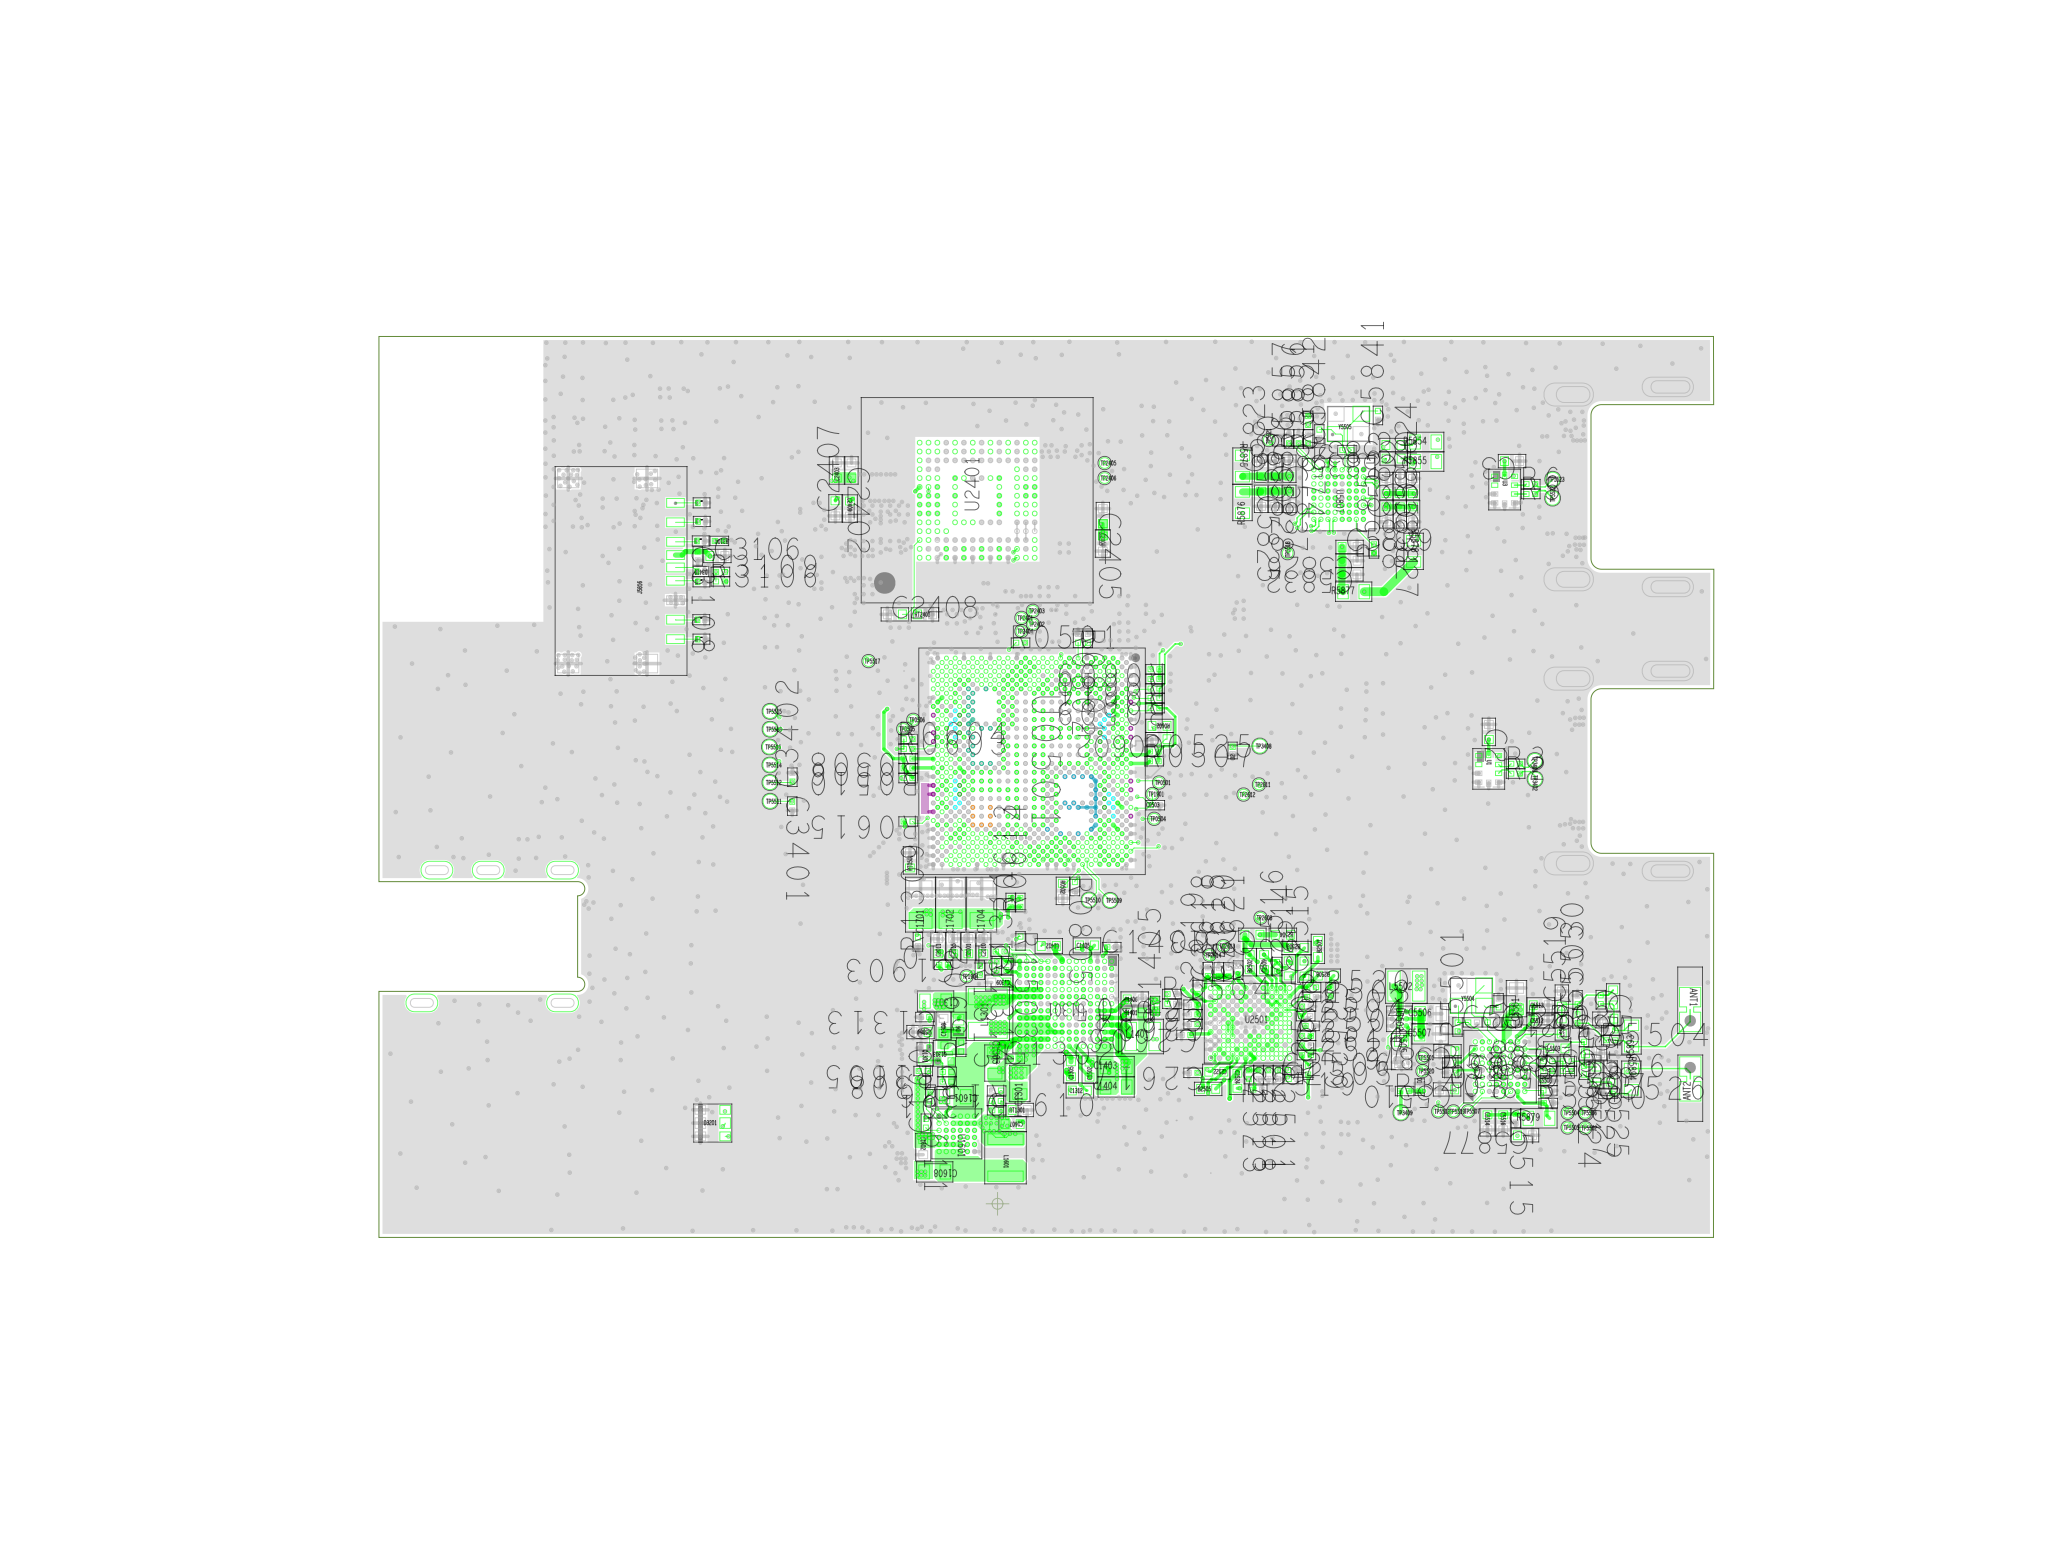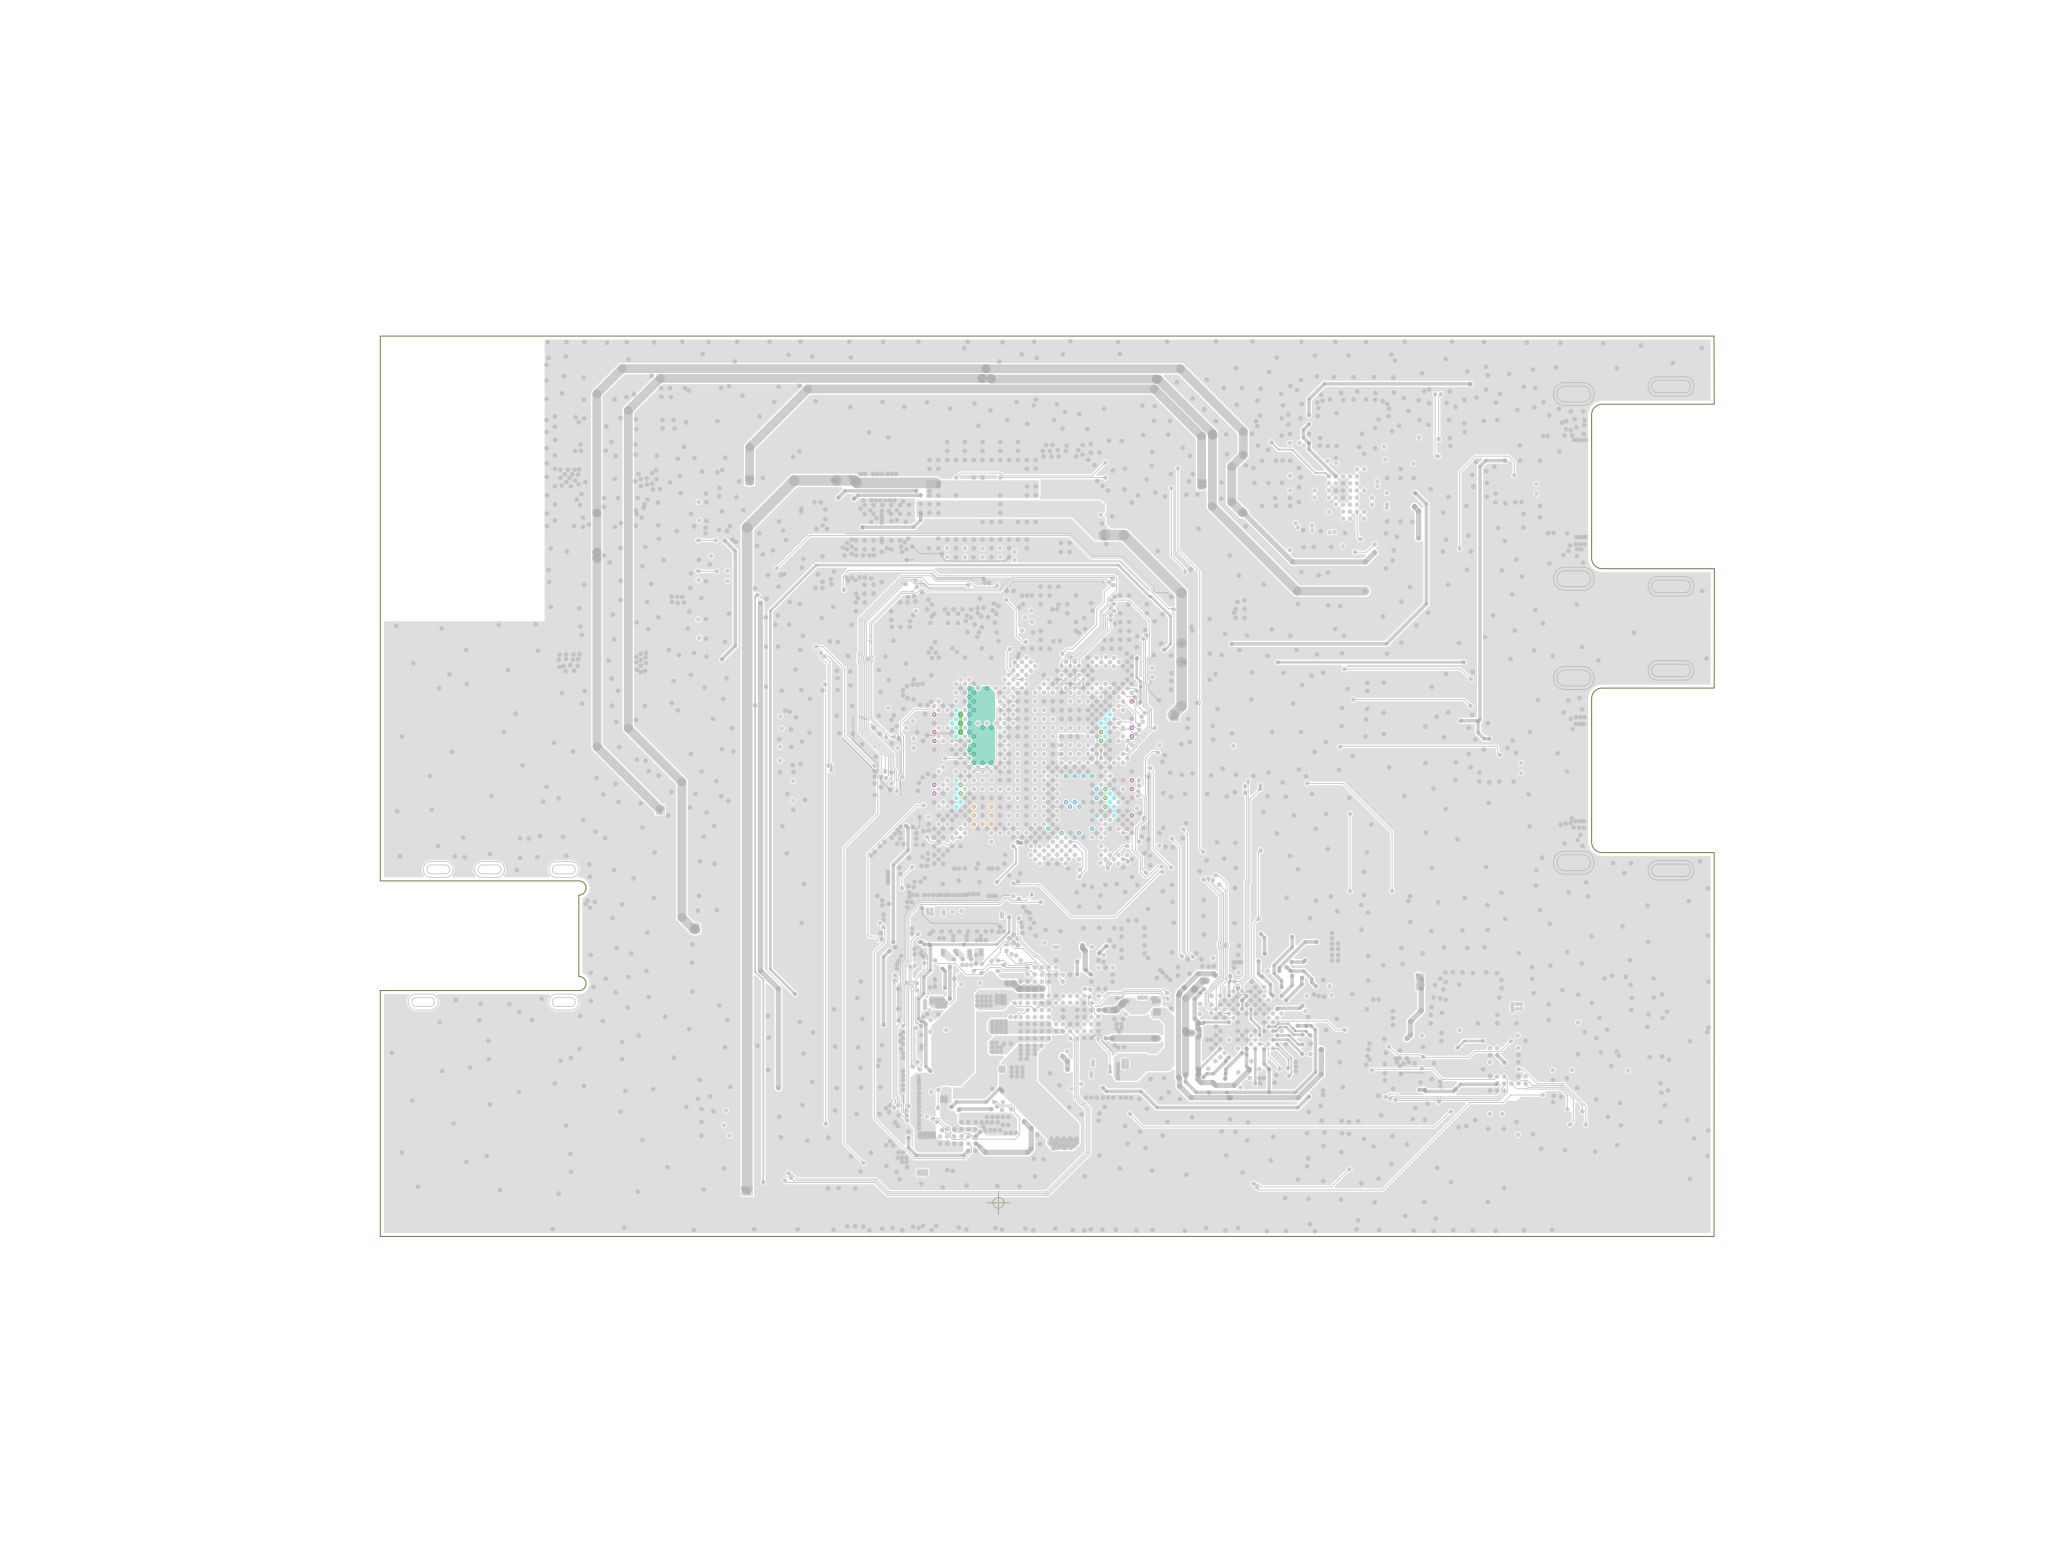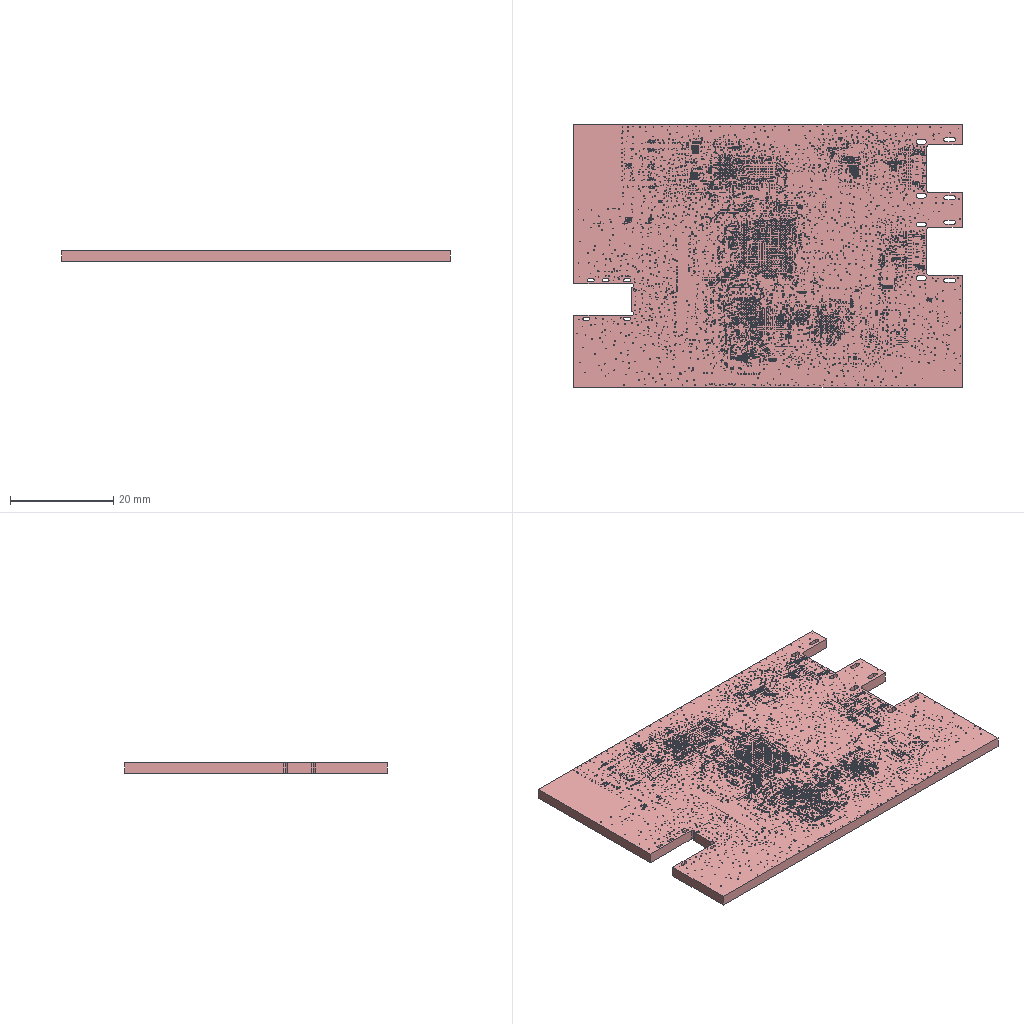Circuit board layout | Cadence Allegro | box 75.4 x 50.9 x 2.1 mm
Layer stack:
# Cadence Allegro layer stack of  (unit mm; from the constraint file cross-section; dielectric type: 0 not recorded (Allegro does not mark core vs prepreg), 3 surface material)
index,name,kind,layer,copper_thickness_mm,dielectric_type,dielectric_thickness_mm,dielectric_material,dielectric_constant
0,Top Surface,other,,,,,,
1,TOP,copper,TOP,0.0305,,,,
2,Dielectric1,dielectric,,,0,0.2032,FR-4,4.5
3,L2,copper,L2,0.0305,,,,
4,Dielectric2,dielectric,,,0,0.2032,FR-4,4.5
5,L3,copper,L3,0.0305,,,,
6,Dielectric3,dielectric,,,0,0.2032,FR-4,4.5
7,L4,copper,L4,0.0305,,,,
8,Dielectric4,dielectric,,,0,0.2032,FR-4,4.5
9,L5,copper,L5,0.0305,,,,
10,Dielectric5,dielectric,,,0,0.2032,FR-4,4.5
11,L6,copper,L6,0.0305,,,,
12,Dielectric6,dielectric,,,0,0.2032,FR-4,4.5
13,L7,copper,L7,0.0305,,,,
14,Dielectric7,dielectric,,,0,0.2032,FR-4,4.5
15,L8,copper,L8,0.0305,,,,
16,Dielectric8,dielectric,,,0,0.2032,FR-4,4.5
17,L9,copper,L9,0.0305,,,,
18,Dielectric9,dielectric,,,0,0.2032,FR-4,4.5
19,BOTTOM,copper,BOTTOM,0.0305,,,,
20,Bottom Surface,other,,,,,,
# drill layer pairs: low layer,high layer
drill_pair,TOP,BOTTOM
drill_pair,L5,BOTTOM
drill_pair,L9,BOTTOM
drill_pair,L2,BOTTOM
drill_pair,L3,BOTTOM
drill_pair,L4,BOTTOM
drill_pair,L6,BOTTOM
drill_pair,L8,BOTTOM
drill_pair,L7,BOTTOM
Part placement, first 475 of 804 lines:
REFDES,COMP_VALUE,SYM_NAME,SYM_X,SYM_Y,SYM_ROTATE,SYM_MIRROR
ANT1,818001475,PIN_ANT_818001475,39.13,11.5,270.000,NO
ANT2,818001475,PIN_ANT_818001475,39.14,6.53,90.000,NO
B301,HZ1005K102TF  1KOHM/100MHZ,FB0402,-23.65,9.9,180.000,YES
B302,HZ1005K102TF  1KOHM/100MHZ,FB0402,-29.6,20.55,270.000,YES
B303,MPZ1608S601AT  600OHM/100MHZ,FB0603_TDK,-24.55,20.25,180.000,YES
B304,HZ1005K102TF 1800ohm,FB0402,-19.1,16.93,180.000,YES
B306,HZ1005K102TF  1KOHM/100MHZ,FB0402,-19.56,15.72,270.000,YES
B2501,BLM15PD121SN1D 120OHM/100MHZ,BLM15AG121SN1D,18.1,14.4,90.000,NO
B2502,HZ1005K102TF  1KOHM/100MHZ,FB0402,14.25,13.65,90.000,NO
B2503,BLM15PD121SN1D 120OHM/100MHZ,BLM15AG121SN1D,16.89,14.45,180.000,NO
B2504,HZ1005K102TF  1KOHM/100MHZ,FB0402,16.12,15.2,180.000,NO
B2505,HZ1005K102TF  1KOHM/100MHZ,FB0402,11.9,6.49,0.000,NO
B2508,BLM15PD121SN1D 120OHM/100MHZ,BLM15AG121SN1D,18.55,12.89,180.000,NO
C2,0.1uF,C0402,27.76,26.66,270.000,NO
C3,0.1uF,C0402,29.07,41.96,180.000,NO
C204,1UF,C0402,28.28,22.49,90.000,YES
C301,470PF,C0201,-20.21,15.97,90.000,YES
C302,DNI(470PF),C0201,-22.5,20.2,90.000,YES
C303,DNI(470PF),C0201,-27.5,20.8,90.000,YES
C304,DNI(33pF),C0402,-21.8,10.3,270.000,YES
C305,DNI(33pF),C0402,-28.15,20.55,90.000,YES
C306,DNI(470PF),C0201,-21.15,10.05,270.000,YES
C307,DNI(33pF),C0402,-17.4,18.18,270.000,YES
C308,DNI(33pF),C0402,-20.3,17.32,270.000,YES
C309,DNI(33pF),C0402,-16.57,18.18,270.000,YES
C310,DNI(33pF),C0402,-16.98,19.4,0.000,YES
C0503,DNI(10nF),C0201,8.91,22.52,0.000,NO
C0602,DNI(82PF),C0402,9.15,26.25,180.000,NO
C0902,1uF,C0201,4.55,29.65,180.000,YES
C0903,1uF,C0201,-1.84,20.45,270.000,YES
C0904,22uf,NFMJMPC226R0G3,4,23.6,90.000,YES
C0905,22uf,NFMJMPC226R0G3,4,22,90.000,YES
C0906,22uf,NFMJMPC226R0G3,5.4,23.6,90.000,YES
C0907,22uf,NFMJMPC226R0G3,5.4,22,270.000,YES
C0913,22UF,0603-BIG,7.85,21.7,270.000,YES
C0914,1uF,C0201,-3.9,28.75,0.000,YES
C0915,1uF,C0201,7.1,29.05,270.000,YES
C0916,1uF,C0201,7,21.05,90.000,YES
C0917,1uF,C0201,-2.95,21.15,90.000,YES
C0918,220NF,C0201,-0.325,27.3,90.000,YES
C0922,22uf,NFMJMPC226R0G3,0.75,26.95,0.000,YES
C0923,22uf,NFMJMPC226R0G3,0.75,28.2,0.000,YES
C0924,22uf,NFMJMPC226R0G3,7.175,27.3,90.000,YES
C0925,22uf,NFMJMPC226R0G3,-3.75,25.45,90.000,YES
C0926,1uF,C0201,7.95,28.35,180.000,YES
C0927,1uF,C0201,7.3,26.15,0.000,YES
C0928,1uF,C0201,7.8,23.9,180.000,YES
C0929,1uF,C0201,7.8,23.35,180.000,YES
C0932,22uf,NFMJMPC226R0G3,-1.85,29.75,0.000,YES
C0933,22uf,NFMJMPC226R0G3,-0.25,29.75,0.000,YES
C0934,22uf,NFMJMPC226R0G3,-1.425,28.3,0.000,YES
C0935,22uf,NFMJMPC226R0G3,-1.375,26.95,0.000,YES
C0936,22uf,NFMJMPC226R0G3,-1.93,25.54,0.000,YES
C0937,22uf,NFMJMPC226R0G3,-0.31,25.53,0.000,YES
C0938,22uf,NFMJMPC226R0G3,-1.3,21.85,270.000,YES
C0939,22uf,NFMJMPC226R0G3,-0.1,21.85,90.000,YES
C0940,1uF,C0201,-0.6,23.15,270.000,YES
C0941,1uF,C0201,-0.05,23.15,270.000,YES
C0942,1uF,C0201,1.75,20.15,0.000,YES
C0944,1uF,C0201,-1.5,24.55,180.000,YES
C1002,1uF,C0201,3.05,29.35,270.000,YES
C1003,1uF,C0201,0.95,20.45,90.000,YES
C1004,1uF,C0201,6,29.6,270.000,YES
C1005,22uf,NFMJMPC226R0G3,-2.95,27.65,90.000,YES
C1006,22uf,NFMJMPC226R0G3,5.4,25.9,0.000,YES
C1010,1uF,C0201,2.2,28.9,0.000,YES
C1012,1uF,C0201,4,20.2,180.000,YES
C1014,1uF,C0201,1.75,20.7,0.000,YES
C1015,22uf,NFMJMPC226R0G3,5.575,27.275,0.000,YES
C1016,22uf,NFMJMPC226R0G3,-2.85,23.55,0.000,YES
C1021,1uF,C0201,-1.75,23.7,90.000,YES
C1022,1uF,C0201,5.45,28.525,90.000,YES
C1023,1uF,C0201,3.75,29.45,270.000,YES
C1025,1uF,C0201,-2.95,29.6,270.000,YES
C1026,1uF,C0201,5,20.75,0.000,YES
C1029,1uF,C0201,-0.35,28.5,90.000,YES
C1030,1uF,C0201,6.43,21.05,90.000,YES
C1031,1uF,C0201,5.375,29.575,270.000,YES
C1032,1uF,C0201,-2.95,22.3,90.000,YES
C1033,1uF,C0201,6.4,22.75,90.000,YES
C1041,1uF,C0201,-2.4,21.15,90.000,YES
C1042,1uF,C0201,-2.8,28.75,0.000,YES
C1043,1uF,C0201,6.7,21.85,180.000,YES
C1044,1uF,C0201,6,28.55,90.000,YES
C1045,220NF,C0201,-2.4,22.3,90.000,YES
C1046,220NF,C0201,6.5,25.9,270.000,YES
C1101,100NF,C0201,1.4,29.7,270.000,YES
C1102,1uF,C0201,0.85,29.7,270.000,YES
C1103,22uf,NFMJMPC226R0G3,2.375,27.925,0.000,YES
C1104,22uf,NFMJMPC226R0G3,1.6,25.1,0.000,YES
C1105,22uf,NFMJMPC226R0G3,1.6,23.7,0.000,YES
C1107,1uF,C0201,-2.55,24.55,0.000,YES
C1108,1uF,C0201,7.05,25.1,180.000,YES
C1109,1uF,C0201,5.85,20.35,90.000,YES
C1110,22uf,NFMJMPC226R0G3,2.35,26.5,0.000,YES
C1111,1uF,C0201,-0.7,20.45,90.000,YES
C1112,1uF,C0201,-0.15,20.45,90.000,YES
C1113,1uF,C0201,0.4,20.45,90.000,YES
C1114,1uF,C0201,2.5,29.7,270.000,YES
C1116,1uF,C0201,-1.5,22.9,180.000,YES
C1117,22uf,NFMJMPC226R0G3,3.75,25.325,90.000,YES
C1118,22uf,NFMJMPC226R0G3,1.54,21.69,0.000,YES
C1119,4.7uF,0402-BIG,4.675,28.6,90.000,YES
C1120,1UF,C0402,3.7,28.15,90.000,YES
C1121,1UF,C0402,5.13,24.94,0.000,YES
C1124,1uF,C0201,-0.3,24.55,180.000,YES
C1125,1uF,C0201,3.65,27,270.000,YES
C1126,1uF,C0201,1.75,22.7,0.000,YES
C1127,22uF,0402-BIG,6,18.65,90.000,YES
C1171,1uF,C0201,6.95,22.75,90.000,YES
C1172,1uF,C0201,6.55,28.6,270.000,YES
C1184,1uF,C0201,-1.2,23.7,90.000,YES
C1185,1uF,C0201,-0.3,24,180.000,YES
C1301,4.7UF,0603-BIG,1.26,6.8,90.000,NO
C1302,DNI(33pF),C0201,1,8.2,0.000,NO
C1303,4.7UF,0603-BIG,-0.15,7.95,270.000,NO
C1305,0.027uf,0402-BIG,4.15,7.6,90.000,NO
C1307,22UF,0603-BIG,-3.5,11.45,180.000,NO
C1308,4.7uF,0402-BIG,-3.05,10.05,90.000,NO
C1309,10uF,0402-BIG,0.1,12.5,180.000,NO
C1310,100NF,C0201,0.15,14.25,180.000,NO
C1311,1uF,C0201,0.5,13.45,90.000,NO
C1312,4.7uF,0402-BIG,4.65,6.4,0.000,NO
C1313,220PF,C0201,-4.1,10.55,180.000,NO
C1314,220PF,C0201,1.95,7.23,0.000,YES
C1315,100NF,C0201,-2.85,7.45,180.000,NO
C1401,2.2uF,0402-BIG,7.75,10.8,0.000,NO
C1403,22UF,0603-BIG,6.7,7.75,0.000,NO
C1404,22UF,0603-BIG,6.7,6.6,0.000,NO
C1405,DNI(10UF),0402-BIG,5.05,14.6,0.000,NO
C1406,2.2uF,0402-BIG,7.75,11.55,0.000,NO
C1409,100NF,C0201,6.45,14.5,0.000,NO
C1412,10uF,0402-BIG,2.896,14.563,180.000,NO
C1502,10uF,0402-BIG,5.2,7.58,90.000,NO
C1503,100NF,C0201,6,11.74,180.000,YES
C1504,1uF,C0201,6.1,11.21,0.000,YES
C1505,100NF,C0201,6.91,9.18,90.000,YES
C1601,4.7UF,0603-BIG,-2.4,6.05,180.000,NO
C1602,10uF,0402-BIG,-4.2,3.2,270.000,NO
C1606,100NF,C0201,-4.05,4.55,90.000,NO
C1607,0.027uf,0402-BIG,0.85,4.5,180.000,NO
C1608,22UF,0603-BIG,-3.55,1.8,180.000,NO
C1610,1uF,C0201,-0.05,5.28,0.000,NO
C1701,47uF,C0805,-4.35,16.9,90.000,NO
C1702,47uF,C0805,-2.65,16.9,90.000,NO
C1703,2.2uF,0402-BIG,2.65,14.68,270.000,YES
C1704,47uF,C0805,-0.9,16.9,90.000,NO
C1705,2.2uF,0402-BIG,1.5,16.61,270.000,YES
C1706,2.2uF,0402-BIG,0.41,16.6,270.000,YES
C1707,2.2uF,0402-BIG,-0.61,16.6,270.000,YES
C1708,2.2uF,0402-BIG,-1.66,16.59,270.000,YES
C1709,2.2uF,0402-BIG,-2.68,16.59,270.000,YES
C1801,2.2uF,0402-BIG,-5.375,13.85,0.000,YES
C1802,2.2uF,0402-BIG,2.65,10,270.000,YES
C1803,22UF,0603-BIG,4.83,6.75,90.000,YES
C1804,22UF,0603-BIG,3.68,6.75,90.000,YES
C1805,2.2uF,0402-BIG,-5.375,14.85,0.000,YES
C1806,2.2uF,0402-BIG,2.65,11.55,270.000,YES
C1807,22UF,0603-BIG,6.04,9.82,90.000,YES
C1808,2.2uF,0402-BIG,2.65,13.13,270.000,YES
C1809,2.2uF,0402-BIG,-5.4,11.775,0.000,YES
C1810,22UF,0603-BIG,-8,8.3,90.000,YES
C1811,22UF,0603-BIG,-9.15,8.3,90.000,YES
C1812,2.2uF,0402-BIG,-5.375,12.8,0.000,YES
C1813,22UF,0603-BIG,-9.45,11.25,90.000,YES
C1814,22UF,0603-BIG,-9.45,13.6,270.000,YES
C1901,47uF,C0805,2.21,5.35,90.000,YES
C1903,100NF,C0201,-3.05,13.5,180.000,NO
C1904,1uF,C0201,-0.63,7.14,90.000,YES
C1905,4.7uF,0402-BIG,-1.09,8.55,90.000,YES
C1906,1000pF,C0402,-3.47,7.06,0.000,YES
C1907,10uF,0402-BIG_H0P9,-1.95,8.55,90.000,YES
C2001,4.7uF,0402-BIG,-1.65,14.55,90.000,NO
C2002,1uF,C0201,-3.1,7.95,180.000,YES
C2003,1uF,C0201,-4.275,8.85,0.000,YES
C2004,4.7uF,0402-BIG,-0.23,8.51,90.000,YES
C2005,4.7uF,0402-BIG,-5.45,8.6,90.000,YES
C2006,4.7uF,0402-BIG,-6.55,8.525,90.000,YES
C2007,4.7uF,0402-BIG,-5.725,10.4,270.000,YES
C2008,4.7uF,0402-BIG,5.85,16.575,270.000,YES
C2009,4.7uF,0402-BIG,0.63,8.51,90.000,YES
C2010,4.7uF,0402-BIG,-0.8,14.55,90.000,NO
C2011,2.2uF,0402-BIG,-3.35,14.55,90.000,NO
C2012,2.2uF,0402-BIG,-4.67,7.06,90.000,YES
C2013,2.2uF,0402-BIG,1.86,7.93,180.000,YES
C2014,2.2uF,0402-BIG,1.86,8.79,180.000,YES
C2015,2.2uF,0402-BIG,-2.5,14.55,90.000,NO
C2016,1uF,C0201,-5.6,7.35,0.000,YES
C2017,1uF,C0201,-4.275,8.3,0.000,YES
C2018,1uF,C0201,-4.95,10,270.000,YES
C2019,DNI(1UF),C0201,-3.1,8.48,180.000,YES
C2020,1uF,C0201,-4.28,16.26,0.000,YES
C2021,1uF,C0201,-3.1,9.05,180.000,YES
C2022,4.7uF,0402-BIG,-5.85,6.62,0.000,YES
C2101,47uF,C0805,12.06,10.45,180.000,YES
C2102,2.2uF,0402-BIG,9.85,13.9,0.000,YES
C2103,47uF,C0805,12.04,12.58,180.000,YES
C2104,100NF,C0201,6.95,12.7,90.000,YES
C2105,2.2uF,0402-BIG,9.84,9.1,0.000,YES
C2106,1UF,C0402,7,11.35,270.000,YES
C2107,2.2uF,0402-BIG,8.27,9.1,0.000,YES
C2108,2.2uF,0402-BIG,8.3,13.9,0.000,YES
C2402,0.1uF,C0402,-8.25,41.43,270.000,NO
C2403,2.2uF,0402-BIG,-9.08,41.43,90.000,NO
C2405,DNI(0.1uF),C0402,5.95,38.85,270.000,NO
C2406,2.2uF,0402-BIG,5.95,37.3,270.000,NO
C2407,DNI(0.1uF),C0402,-9.16,39.29,90.000,NO
C2408,DNI(0.1uF),C0402,-5.8,33.3,0.000,NO
C2409,2.2uF,0402-BIG,-8.34,39.28,270.000,NO
C2501,100NF,C0201,15.3,7.3,270.000,NO
C2502,DNI(330PF),C0201,17.45,11.15,0.000,NO
C2503,DNI(680pf),C0201,17.74,11.69,0.000,NO
C2504,DNI(680pf),C0201,17.41,10.6,0.000,NO
C2505,DNI(100pf),C0201,16.7,7.05,0.000,NO
C2506,DNI(100pf),C0201,16.65,7.56,0.000,NO
C2507,100NF,C0201,17.65,10.05,0.000,NO
C2509,4.7uF,0402-BIG,15.06,13.65,90.000,NO
C2511,470nF,C0201,15.85,7.3,270.000,NO
C2513,1UF,C0402,14.4,15.2,180.000,NO
C2514,470nf,C0402,16.45,13.3,90.000,NO
C2515,470nf,C0402,17.34,13.29,90.000,NO
C2516,1uF,C0201,15.8,13.4,90.000,NO
C2518,100NF,C0201,14.75,7.3,270.000,NO
C2519,100NF,C0201,14.7,6.45,0.000,NO
C2520,470nF,C0201,17.74,12.23,0.000,NO
C2521,1uF,C0201,17.45,9.49,0.000,NO
C2522,4.7uF,0402-BIG,12.36,7.46,180.000,NO
C2523,1uF,C0201,14.2,7.3,270.000,NO
C2524,4.7uF,0402-BIG,13.55,6.95,270.000,NO
C2527,100NF,C0201,17.45,8.4,0.000,NO
C2529,470nF,C0201,18.82,11.97,270.000,NO
C2601,100NF,C0201,11.05,11.25,180.000,NO
C2603,100NF,C0201,11.05,10.15,180.000,NO
C2606,100NF,C0201,10.65,9.54,180.000,NO
C2614,100NF,C0201,11.05,10.7,180.000,NO
C2615,100NF,C0201,12.5,13.1,90.000,NO
C2616,100NF,C0201,17.45,8.95,0.000,NO
C2617,100NF,C0201,11.05,7.4,180.000,NO
C2618,100NF,C0201,11.88,13.11,90.000,NO
C2619,100NF,C0201,11.3,12.1,90.000,NO
C2620,100NF,C0201,13.05,13.1,90.000,NO
C2621,100NF,C0201,13.6,13.2,90.000,NO
C3106,33pF,C0402,-15.83,36.6,0.000,NO
C3108,1uF,C0201,-16.94,36.6,270.000,NO
C3307,100NF,C0201,28.24,26.55,0.000,YES
C3308,100NF,C0201,28.24,27.09,0.000,YES
C3317,100NF,C0201,28.18,20.71,0.000,YES
C3318,100NF,C0201,28.18,21.25,0.000,YES
C3320,100pF,C0201,27.05,18.24,180.000,YES
C3321,100NF,C0201,24.09,29.57,180.000,YES
C3322,100NF,C0201,24.09,29.01,180.000,YES
C3323,DNI(1UF),C0402,26.55,27.25,0.000,YES
C3401,10nF,C0201,-11.6,22.47,270.000,NO
C3402,10nF,C0201,-11.59,24.1,90.000,NO
C5301,DNI(100pf),C0201,0.83,44.7,0.000,YES
C5302,2.2uF,0402-BIG,-2.5,39.1,180.000,YES
C5303,56pF,C0201,-2.3,37.8,180.000,YES
C5307,DNI(22UF),0603-BIG,-3.35,36.95,180.000,YES
C5308,10nF,C0201,-6.35,44.4,270.000,YES
C5309,10nF,C0201,-6.95,38.85,270.000,YES
C5310,100pF,C0201,-5.35,45.5,90.000,YES
C5311,DNI(10UF),0402-BIG,-7.55,37,0.000,YES
C5312,4.7uF,0402-BIG,-7.55,37.75,0.000,YES
C5313,10nF,C0201,-7.5,38.65,270.000,YES
C5314,100pF,C0201,-5.3,38.85,270.000,YES
C5315,10nF,C0201,-6.15,38.55,180.000,YES
C5316,DNI(4.7UF),0402-BIG,-4.15,37.9,180.000,YES
C5317,470nF,C0201,-3.65,38.85,90.000,YES
C5318,10nF,C0201,-5.8,44.4,270.000,YES
C5319,DNI(10UF),0402-BIG,-2.85,45.25,270.000,YES
C5320,4.7uF,0402-BIG,-6.55,45.75,270.000,YES
C5321,10nF,C0201,-7.2,45.5,270.000,YES
C5322,DNI(10UF),0402-BIG,-6.4,37.3,90.000,YES
C5323,470nF,C0201,-4.8,45.5,270.000,YES
C5324,220NF,C0201,-2.8,39.9,180.000,YES
C5325,10nF,C0201,-2.8,40.45,180.000,YES
C5326,10nF,C0201,-7.2,44.7,0.000,YES
C5327,10nF,C0201,-2.8,43.65,180.000,YES
C5328,470nF,C0201,-6.15,39.1,180.000,YES
C5329,10nF,C0201,-7.2,44.15,0.000,YES
C5330,10nF,C0201,-5.25,44.4,270.000,YES
C5331,DNI(10nF),C0201,-4.15,44.4,270.000,YES
C5332,DNI(100NF),C0201,-2.8,44.2,180.000,YES
C5333,10nF,C0201,-3.6,44.4,270.000,YES
C5340,22pF,C0201,-3.1,38.05,90.000,YES
C5501,4.7UF,0603-BIG,29.32,11.59,90.000,NO
C5502,100NF,C0201,29.06,10.25,0.000,NO
C5505,22UF,0603-BIG,22.83,8.6,270.000,NO
C5506,10uF,0603-BIG,24.47,10.74,0.000,NO
C5507,10uF,0603-BIG,24.44,9.6,0.000,NO
C5508,100NF,C0201,31.09,6.95,0.000,NO
C5510,1UF,C0402,25.4,6.46,180.000,NO
C5512,2.2uF,0402-BIG,30.68,10.35,0.000,NO
C5513,2.2uF,0402-BIG,30.69,11.22,0.000,NO
C5514,2.2uF,0402-BIG,27.68,4.6,270.000,NO
C5515,470nF,C0201,29.28,4.84,270.000,NO
C5516,2.2uF,0402-BIG,28.57,4.6,270.000,NO
C5518,18pF,C0402,34.78,11.66,270.000,NO
C5519,560pF,C0402,31.88,11.59,90.000,NO
C5520,150pF,C0201,34.08,11.53,270.000,NO
C5521,15pF,C0402,34.4,10.46,180.000,NO
C5522,330PF,C0201,34.65,9.79,180.000,NO
C5523,560pF,C0402,33.64,8.5,180.000,NO
C5524,150pF,C0201,33.14,7.55,270.000,NO
C5525,15pF,C0402,34.64,7.3,270.000,NO
C5526,330PF,C0201,34.49,6.22,0.000,NO
C5527,18pF,C0402,33.84,7.3,270.000,NO
C5528,18PF,C0201,26.84,10.25,0.000,NO
C5529,18PF,C0201,27.94,10.25,0.000,NO
C5530,1nF,C0201,31.09,7.5,180.000,NO
C5531,1nF,C0201,31.09,8.05,180.000,NO
C5550,220PF,C0201,32.77,11.52,90.000,NO
C5551,220PF,C0201,33.14,9.4,270.000,NO
C5701,DNI(8.2nH),L0201,-23.44,45.16,270.000,YES
C5702,DNI(2.2pF),C0201,-21.71,45.17,270.000,YES
C5708,4.7uF,0402-BIG,-9.95,42.2,180.000,YES
C5709,10pF,C0201,-12.72,42.04,90.000,YES
C5710,10pF,C0201,-12.15,42.05,90.000,YES
C5711,100NF,C0201,-11,42.05,90.000,YES
C5712,100NF,C0201,-11.55,42.05,90.000,YES
C5716,18PF,C0201,-8.05,44.25,270.000,YES
C5822,1UF,C0402,28.44,41.22,270.000,YES
C5823,1NF,C0402,14.89,41.53,90.000,NO
C5824,1NF,C0402,23.47,40.55,90.000,NO
C5825,1NF,C0402,14.89,39.83,270.000,NO
C5826,1UF,C0402,19.89,36.33,180.000,NO
C5827,1NF,C0402,22.73,38.95,270.000,NO
C5828,0.1uF,C0402,15.69,41.53,270.000,NO
C5830,0.1uF,C0402,15.69,39.83,90.000,NO
C5831,0.1uF,C0402,22.72,40.55,270.000,NO
C5832,0.1uF,C0402,19.88,35.56,180.000,NO
C5833,0.1uF,C0402,21.97,38.95,90.000,NO
C5834,0.1uF,C0402,22.37,42.87,180.000,NO
C5835,0.1uF,C0402,22.38,42.1,180.000,NO
C5836,1UF,C0402,16.49,39.83,90.000,NO
C5837,1UF,C0402,16.49,41.53,270.000,NO
C5838,1UF,C0402,21.97,40.55,270.000,NO
C5839,1NF,C0402,19.89,37.11,0.000,NO
C5840,1UF,C0402,23.48,38.95,90.000,NO
C5841,18PF,C0201,21.49,44.54,90.000,NO
C5842,18PF,C0201,18.18,43.49,90.000,NO
C5849,1uF,C0201,-21.52,40.09,90.000,YES
C5850,100NF,C0201,-22.12,40.09,90.000,YES
C5852,100NF,C0201,-20.92,40.09,90.000,YES
C5855,4.7UF,0603-BIG,16.7,45.77,270.000,YES
C5856,4.7UF,0603-BIG,18.84,42.79,90.000,YES
C5857,4.7UF,0603-BIG,20.05,42.78,90.000,YES
C5858,10uF,0603-BIG,17.62,42.79,90.000,YES
C5859,10pF,C0201,-11.8,36.9,90.000,YES
C5860,100NF,C0201,-10.7,36.9,90.000,YES
C5861,DNI(8.2nH),L0201,-23.49,37.97,270.000,YES
C5862,100NF,C0201,-11.25,36.9,90.000,YES
C5863,10pF,C0201,-12.35,36.9,90.000,YES
C5864,DNI(2.2pF),C0201,-21.69,37.97,270.000,YES
C5866,18PF,C0201,-8.25,41.2,0.000,YES
C5867,4.7uF,0402-BIG,-9.6,37.15,270.000,YES
C5870,100NF,C0201,28.05,37.15,0.000,YES
C5871,100NF,C0201,28.05,36.61,0.000,YES
C5872,100NF,C0201,28.09,42.99,0.000,YES
C5873,100NF,C0201,28.09,42.45,0.000,YES
C5876,220NF,C0402,25.42,8.62,180.000,NO
C5877,470nf,C0402,29.8,3.87,180.000,NO
C5878,DNI(100NF),C0201,-22.79,42.23,270.000,YES
C5879,DNI(100NF),C0201,-22.78,41.03,90.000,YES
C5880,18PF,C0201,-9.25,45.1,0.000,YES
C5881,18PF,C0201,-9.7,40.25,90.000,YES
C5882,6.8PF,C0201,-13.9,38.75,0.000,YES
C5883,6.8PF,C0201,-13.65,43.85,0.000,YES
C5884,9pF,C0201,0.78,41.92,0.000,YES
C5885,9pF,C0201,-0.25,44.7,0.000,YES
C5886,47PF,C0201,-24.39,37.72,0.000,YES
C5887,47PF,C0201,-25.65,35.1,0.000,YES
C5888,47PF,C0201,-24.28,44.88,0.000,YES
C5889,47PF,C0201,-25.69,47.76,0.000,YES
D1,ESD7181MUT5G,X3DFN2_0P62X0P32_0P43_0P355,23.85,6.59,270.000,NO
D2,ESD7181MUT5G,X3DFN2_0P62X0P32_0P43_0P355,13.28,25.61,90.000,NO
D3,ESD7181MUT5G,X3DFN2_0P62X0P32_0P43_0P355,-29.82,24.2,270.000,YES
D4,ESD7181MUT5G,X3DFN2_0P62X0P32_0P43_0P355,-25.17,24.14,270.000,YES
D5,ESD7181MUT5G,X3DFN2_0P62X0P32_0P43_0P355,-20.74,24.1,270.000,YES
D6,NSR05F40NXT5G,DSN2,-2.2,10.1,90.000,NO
D201,PTVS15VU1UPA,DFN2020-3,25.99,22.81,270.000,YES
D202,PESD5V0H1BSF,DSN0603-2,30.33,24.81,180.000,YES
D203,PESD5V0H1BSF,DSN0603-2,30.33,25.99,180.000,YES
D204,PESD5V0H1BSF,DSN0603-2,30.33,24.22,180.000,YES
D212,PESD5V0H1BSF,DSN0603-2,30.33,25.41,180.000,YES
D213,PESD5V0H1BSF,DSN0603-2,30.32,22.47,180.000,YES
D214,PESD5V0H1BSF,DSN0603-2,30.32,21.29,180.000,YES
D215,PESD5V0H1BSF,DSN0603-2,30.32,21.88,180.000,YES
D216,PESD5V0H1BSF,DSN0603-2,30.32,20.71,180.000,YES
D217,PESD5V0H1BSF,DSN0603-2,30.33,23.63,180.000,YES
D218,PESD5V0H1BSF,DSN0603-2,30.32,23.05,180.000,YES
D220,PESD5V0H1BSF,DSN0603-2,30.33,27.12,180.000,YES
D222,PESD5V0H1BSF,DSN0603-2,30.33,26.57,180.000,YES
D223,PESD5V0H1BSF,DSN0603-2,30.34,27.71,180.000,YES
D224,PESD5V0H1BSF,DSN0603-2,30.34,28.26,180.000,YES
D301,PESD5V0F1BRSF,DSN0603-2,-20.21,14.42,270.000,YES
D304,VESD5451Z-2/TR,DFN0603-2L,-22.5,9.95,90.000,YES
D305,VESD5451Z-2/TR,DFN0603-2L,-28.85,20.75,270.000,YES
D306,VESD5451Z-2/TR,DFN0603-2L,-18,16.85,270.000,YES
D3101,DNI(PESD5V0H1BSF),DSN0603-2,-16.71,38.55,180.000,NO
D3102,DNI(PESD5V0H1BSF),DSN0603-2,-16.73,31.9,180.000,NO
D3105,DNI(PESD5V0H1BSF),DSN0603-2,-16.77,37.45,180.000,NO
D3107,DNI(PESD5V0H1BSF),DSN0603-2,-16.73,35.14,180.000,NO
D3111,DNI(PESD5V0H1BSF),DSN0603-2,-16.74,33,180.000,NO
D3112,DNI(PESD5V0H1BSF),DSN0603-2,-16.72,39.6,180.000,NO
D3201,19-337-R6GHBHC-A01-2T,19-337-R6GHBHC-A01-2T,-16.09,4.56,0.000,NO
D3403,PTVS15VU1UPA,DFN2020-3,26.94,40.85,180.000,YES
D3404,PESD5V0H1BSF,DSN0603-2,30.21,37.18,180.000,YES
D3405,PESD5V0H1BSF,DSN0603-2,30.21,36.6,180.000,YES
D3406,PESD5V0H1BSF,DSN0603-2,30.21,38.35,180.000,YES
D3407,PESD5V0H1BSF,DSN0603-2,30.21,37.76,180.000,YES
D3408,PESD5V0H1BSF,DSN0603-2,30.21,41.23,180.000,YES
D3409,PESD5V0H1BSF,DSN0603-2,30.21,41.82,180.000,YES
D3410,PESD5V0H1BSF,DSN0603-2,30.21,40.65,180.000,YES
D3411,PESD5V0H1BSF,DSN0603-2,30.21,40.08,180.000,YES
D3412,PESD5V0H1BSF,DSN0603-2,30.21,42.98,180.000,YES
D3413,PESD5V0H1BSF,DSN0603-2,30.21,42.39,180.000,YES
D3414,PESD5V0H1BSF,DSN0603-2,30.21,44.16,180.000,YES
D3415,PESD5V0H1BSF,DSN0603-2,30.21,43.57,180.000,YES
D3416,PESD5V0H1BSF,DSN0603-2,30.21,39.5,180.000,YES
D3417,PESD5V0H1BSF,DSN0603-2,30.21,38.92,180.000,YES
D3418,PMEG3030BEP,SOD128,23.65,42.71,90.000,YES
D3419,VESD5451Z-2/TR,DFN0603-2L,-16.76,35.72,180.000,NO
D3420,VESD5451Z-2/TR,DFN0603-2L,-23.1,20.3,270.000,YES
FIL5804,NFP0QHB372HS2D,NFP0QHBXXXHS2X,29.29,28.02,180.000,YES
FIL5809,NFP0QHB372HS2D,NFP0QHBXXXHS2X,29.15,42.72,180.000,YES
FIL5810,NFP0QHB372HS2D,NFP0QHBXXXHS2X,29.17,36.88,180.000,YES
FIL5811,NFP0QHB372HS2D,NFP0QHBXXXHS2X,29.16,38.05,180.000,YES
FIL5812,NFP0QHB372HS2D,NFP0QHBXXXHS2X,29.15,43.89,180.000,YES
FL205,NFP0QHB372HS2D,NFP0QHBXXXHS2X,29.29,26.83,180.000,YES
FL5703,DEA105150HT-8044A1,DEA105150HT-8044A1,-8.9,43.4,0.000,YES
FL5803,NFP0QHB372HS2D,NFP0QHBXXXHS2X,29.25,20.99,180.000,YES
FL5805,NFP0QHB372HS2D,NFP0QHBXXXHS2X,29.25,22.13,180.000,YES
FL5808,DEA105150HT-8044A1,DEA105150HT-8044A1,-8.85,39.05,90.000,YES
J1,SD-105435,USB_SD-105435,32.52,24.45,90.000,YES
J4601,GB701-8S-H06,PWC_GB701-8S-H06,-29.51,4.52,0.000,YES
J5702,MM8030-2610,RF_MM8030-2610,-19.83,44.91,270.000,YES
J5812,SD-105435,USB_SD-105435,32.52,40.5,90.000,YES
J5814,MM8030-2610,RF_MM8030-2610,-19.86,37.71,270.000,YES
J5816,TF006-17112A91,TF_TF006-17116A91,-18.195,35.75,90.000,NO
J5817,0919 Audio Jack,HP_0919_AUDIO_JACK,-34.775,15.1,180.000,YES
J5818,818001475,PIN_ANT_818001475,-31.68,44.88,0.000,YES
J5819,818001475,PIN_ANT_818001475,-31.57,37.68,0.000,YES
J5820,818001475,PIN_ANT_818001475,-31.63,47.78,0.000,YES
J5821,818001475,PIN_ANT_818001475,-31.65,35.11,0.000,YES
K1,EVPAWBA2AT01,KEY_EVPAWBA2AT01,-29.8,28.24,90.000,YES
K2,EVPAWBA2AT01,KEY_EVPAWBA2AT01,-25.09,28.26,90.000,YES
K3,EVPAWBA2AT01,KEY_EVPAWBA2AT01,-20.5,28.26,90.000,YES
L302,85nH,L0603_LQW18CNR33J00D,-18.6,14.25,180.000,YES
L1301,1uH,L2520_MEKK2520,-0.55,10.75,90.000,NO
L1401,0.47UH,L2016_MEKK2016,8.2,9.45,0.000,NO
L1601,1.0uH,L2520_TFM252008GHM,0.45,2.6,270.000,NO
L1701,0.47UH,L2016_MEKK2016,4.27,14.7,180.000,YES
L1702,0.47UH,L2016_MEKK2016,4.2,16.7,180.000,YES
L1703,0.47UH,L2016_MEKK2016,1.4,18.575,270.000,YES
L1704,0.47UH,L2016_MEKK2016,-0.575,18.575,270.000,YES
L1705,0.47UH,L2016_MEKK2016,-2.525,18.575,270.000,YES
L1706,0.47UH,L2016_MEKK2016,-4.475,18.525,270.000,YES
L1801,0.47UH,L2016_MEKK2016,-7.45,14.25,0.000,YES
L1802,0.47UH,L2016_MEKK2016,4.27,8.77,180.000,YES
L1803,0.47UH,L2016_MEKK2016,-7.15,16.8,270.000,YES
L1804,0.47UH,L2016_MEKK2016,4.27,10.75,180.000,YES
L1805,0.47UH,L2016_MEKK2016,4.27,12.72,180.000,YES
L1806,0.47UH,L2016_MEKK2016,-7.45,10.4,0.000,YES
L1807,0.47UH,L2016_MEKK2016,-7.45,12.35,0.000,YES
L2101,0.47UH,L2016_MEKK2016,10.74,15.51,270.000,YES
L2102,0.47UH,L2016_MEKK2016,10.04,7.48,90.000,YES
L2103,0.47UH,L2016_MEKK2016,8.07,7.48,90.000,YES
L2104,0.47UH,L2016_MEKK2016,8.78,15.51,270.000,YES
L5501,160nH,L0402_H0P7,31.88,10.02,90.000,NO
L5502,1uH,L2016_WPN201610V,23.1,12.3,0.000,NO
L5503,160nH,L0402_H0P7,31.63,8.78,0.000,NO
L5702,DNI(1.7NH),L0201,-14.46,43.59,90.000,YES
L5703,DNI(1.7NH),L0201,-15.02,44.65,90.000,YES
Pad and via stacks, first 103 of 174 lines:
# Allegro (Cadence) via spans and padstacks; design units: ("millimeters" 4 10000)
# via spans: padstack,start_layer,end_layer,net_example,count
VIA0075-02-5-B,ETCH/L5,ETCH/BOTTOM,GND,249
VIA0075-02-9-B,ETCH/L9,ETCH/BOTTOM,GND,891
VIA0075-02-2-B,ETCH/L2,ETCH/BOTTOM,REF_BYP,9
VIA0075-02-3-B,ETCH/L3,ETCH/BOTTOM,GND,2
VIA0075-02-4-B,ETCH/L4,ETCH/BOTTOM,PHONE_ON_N,42
VIA0075-02-6-B,ETCH/L6,ETCH/BOTTOM,CDC_HPH_R,155
VIA0075-02-8-B,ETCH/L8,ETCH/BOTTOM,N369687,392
VIA0075-02-7-B,ETCH/L7,ETCH/BOTTOM,GND,1245
VIA0075-02-T-B,ETCH/TOP,ETCH/BOTTOM,GND,544
# Allegro padstack definitions: name,start_layer,end_layer,drill,plating,holeType,type
VIA0P1X0P25,"ETCH/TOP","ETCH/BOTTOM",0.1,"PLATED","circle_drill","through"
VIA0P2X0P4,"ETCH/TOP","ETCH/BOTTOM",0.2,"PLATED","circle_drill","through"
L9-BOTTOM,"ETCH/L9","ETCH/BOTTOM",0.1,"PLATED","circle_drill","bbvia"
L1-L10,"ETCH/TOP","ETCH/BOTTOM",0.2,"PLATED","circle_drill","through"
0P28X0P3SMD,"ETCH/TOP","ETCH/TOP",0.0,"PLATED","none","smd"
0P24X0P32SMD-OB0P19X0P27PASTE,"ETCH/TOP","ETCH/TOP",0.0,"PLATED","none","smd"
0P5SSMD,"ETCH/TOP","ETCH/TOP",0.0,"PLATED","none","smd"
0P37X0P5SMD,"ETCH/TOP","ETCH/TOP",0.0,"PLATED","none","smd"
0P4X0P7SMD_NP,"ETCH/TOP","ETCH/TOP",0.0,"PLATED","none","smd"
0P4X0P5SMD,"ETCH/TOP","ETCH/TOP",0.0,"PLATED","none","smd"
0P45X0P53SMD,"ETCH/TOP","ETCH/TOP",0.0,"PLATED","none","smd"
0P23X0P65SMD_CONNECTOR,"ETCH/TOP","ETCH/TOP",0.0,"PLATED","none","smd"
0P5X1P6SMD,"ETCH/TOP","ETCH/TOP",0.0,"PLATED","none","smd"
0P55X0P6SMD,"ETCH/TOP","ETCH/TOP",0.0,"PLATED","none","smd"
1P48X2P0SMD-NP,"ETCH/TOP","ETCH/TOP",0.0,"NON_PLATED","none","smd"
0P1CSMD-NSOLDER-NP,"ETCH/TOP","ETCH/TOP",0.0,"PLATED","none","smd"
0P4X1P4SMD,"ETCH/TOP","ETCH/TOP",0.0,"PLATED","none","smd"
0P45X1P4SMD,"ETCH/TOP","ETCH/TOP",0.0,"PLATED","none","smd"
P0P6X1P7OB1P4X2P9R,"ETCH/TOP","ETCH/BOTTOM",0.6,"PLATED","oval slot","through"
P0P6X1P7OB1P25X2P9R,"ETCH/TOP","ETCH/BOTTOM",0.6,"PLATED","oval slot","through"
0P45X0P5SMD,"ETCH/TOP","ETCH/TOP",0.0,"PLATED","none","smd"
0P6X0P8SMD,"ETCH/TOP","ETCH/TOP",0.0,"PLATED","none","smd"
0P45XOP95SMD,"ETCH/TOP","ETCH/TOP",0.0,"PLATED","none","smd"
0P35X2P3SMD,"ETCH/TOP","ETCH/TOP",0.0,"PLATED","none","smd"
0P35X1P3SMD,"ETCH/TOP","ETCH/TOP",0.0,"PLATED","none","smd"
2P0CSMD_NP,"ETCH/TOP","ETCH/TOP",0.0,"PLATED","none","smd"
0P1CSMD,"ETCH/TOP","ETCH/TOP",0.0,"PLATED","none","smd"
0P2X0P6SMD,"ETCH/TOP","ETCH/TOP",0.0,"PLATED","none","smd"
0P2X0P4SMD,"ETCH/TOP","ETCH/TOP",0.0,"PLATED","none","smd"
0P2CSMD,"ETCH/TOP","ETCH/TOP",0.0,"PLATED","none","smd"
1P1X1P3SMD,"ETCH/TOP","ETCH/TOP",0.0,"PLATED","none","smd"
1P0CSMD_NP,"ETCH/TOP","ETCH/TOP",0.0,"PLATED","none","smd"
R0P6X0P8,"ETCH/TOP","ETCH/TOP",0.0,"PLATED","none","smd"
R0P75X1P0,"ETCH/TOP","ETCH/TOP",0.0,"PLATED","none","smd"
R0P24X0P32_PMOB0P19X0P27,"ETCH/TOP","ETCH/TOP",0.0,"PLATED","none","smd"
PIN_ANT,"ETCH/TOP","ETCH/TOP",0.0,"PLATED","none","smd"
SQ0P5,"ETCH/TOP","ETCH/TOP",0.0,"PLATED","none","smd"
R0P45X0P5,"ETCH/TOP","ETCH/TOP",0.0,"PLATED","none","smd"
R0P9X1P3,"ETCH/TOP","ETCH/TOP",0.0,"PLATED","none","smd"
R0P28X0P3,"ETCH/TOP","ETCH/TOP",0.0,"PLATED","none","smd"
R0P3X0P31,"ETCH/TOP","ETCH/TOP",0.0,"PLATED","none","smd"
R0P4X0P5_PMR0P4X0P5_SMR0P5X0P6,"ETCH/TOP","ETCH/TOP",0.0,"PLATED","none","smd"
DFN2020-3,"ETCH/TOP","ETCH/TOP",0.0,"PLATED","none","smd"
R0P5X0P6,"ETCH/TOP","ETCH/TOP",0.0,"PLATED","none","smd"
SQ0P6,"ETCH/TOP","ETCH/TOP",0.0,"PLATED","none","smd"
R0P65X0P8_0P75X0P9_0P55X0P7,"ETCH/TOP","ETCH/TOP",0.0,"PLATED","none","smd"
R0P8X1P05_0P9X1P15_0P7X0P95,"ETCH/TOP","ETCH/TOP",0.0,"PLATED","none","smd"
SQ0P6_SMR0P63X0P65,"ETCH/TOP","ETCH/TOP",0.0,"PLATED","none","smd"
R0P47X0P6_SMR0P5X0P65,"ETCH/TOP","ETCH/TOP",0.0,"PLATED","none","smd"
R0P23X0P3,"ETCH/TOP","ETCH/TOP",0.0,"PLATED","none","smd"
R0P3X0P9,"ETCH/TOP","ETCH/TOP",0.0,"PLATED","none","smd"
PTH_OB0P7X2P2OB1P1X2P9_OFFSET,"ETCH/TOP","ETCH/BOTTOM",0.7,"PLATED","oval slot","through"
PTH_OB0P9X1P9OB1P3X2P8_OFFSET,"ETCH/TOP","ETCH/BOTTOM",0.9,"PLATED","oval slot","through"
R0P3X0P8,"ETCH/TOP","ETCH/TOP",0.0,"PLATED","none","smd"
R0P3X0P7,"ETCH/TOP","ETCH/TOP",0.0,"PLATED","none","smd"
PTH_OB0P6X1P7OB1P1X2P2,"ETCH/TOP","ETCH/BOTTOM",0.6,"PLATED","oval slot","through"
PTH_OB0P6X1P2OB1P1X1P7,"ETCH/TOP","ETCH/BOTTOM",0.6,"PLATED","oval slot","through"
PTH_OB0P5X1P39OB1P0X1P59,"ETCH/TOP","ETCH/BOTTOM",0.5,"PLATED","oval slot","through"
PTH_OB0P6X1P8OB1P0X2P2,"ETCH/TOP","ETCH/BOTTOM",0.6,"PLATED","oval slot","through"
SQ0P35,"ETCH/TOP","ETCH/TOP",0.0,"PLATED","none","smd"
R0P55X0P8,"ETCH/TOP","ETCH/TOP",0.0,"PLATED","none","smd"
R0P24X0P55,"ETCH/TOP","ETCH/TOP",0.0,"PLATED","none","smd"
R0P5X0P55,"ETCH/TOP","ETCH/TOP",0.0,"PLATED","none","smd"
R0P65X0P8,"ETCH/TOP","ETCH/TOP",0.0,"PLATED","none","smd"
R0P24X0P65,"ETCH/TOP","ETCH/TOP",0.0,"PLATED","none","smd"
R0P4X0P5_PM0P4X0P4,"ETCH/TOP","ETCH/TOP",0.0,"PLATED","none","smd"
RF_MM8030-2160_1,"ETCH/TOP","ETCH/TOP",0.0,"PLATED","none","smd"
RF_MM8030-2160_2,"ETCH/TOP","ETCH/TOP",0.0,"PLATED","none","smd"
R1P05X1P2,"ETCH/TOP","ETCH/TOP",0.0,"PLATED","none","smd"
R0P5X1P0,"ETCH/TOP","ETCH/TOP",0.0,"PLATED","none","smd"
PTH_OB0P5X1P3OB1P0X1P8,"ETCH/TOP","ETCH/BOTTOM",0.5,"PLATED","oval slot","through"
R0P55X1P5_NP,"ETCH/TOP","ETCH/TOP",0.0,"PLATED","none","smd"
R0P9X2P2,"ETCH/TOP","ETCH/TOP",0.0,"NON_PLATED","none","smd"
R0P65X1P6,"ETCH/TOP","ETCH/TOP",0.0,"PLATED","none","smd"
R0P6X2P0,"ETCH/TOP","ETCH/TOP",0.0,"PLATED","none","smd"
R0P7X1P7,"ETCH/TOP","ETCH/TOP",0.0,"PLATED","none","smd"
R0P2X0P43,"ETCH/TOP","ETCH/TOP",0.0,"PLATED","none","smd"
R0P41X0P55,"ETCH/TOP","ETCH/TOP",0.0,"PLATED","none","smd"
R0P4X0P45,"ETCH/TOP","ETCH/TOP",0.0,"PLATED","none","smd"
R0P9X1P44,"ETCH/TOP","ETCH/TOP",0.0,"PLATED","none","smd"
R1P2X1P44,"ETCH/TOP","ETCH/TOP",0.0,"PLATED","none","smd"
C0P6_NP,"ETCH/TOP","ETCH/TOP",0.0,"PLATED","none","smd"
C0P8_NP,"ETCH/TOP","ETCH/TOP",0.0,"PLATED","none","smd"
C0P23,"ETCH/TOP","ETCH/TOP",0.0,"PLATED","none","smd"
R0P25X0P35,"ETCH/TOP","ETCH/TOP",0.0,"PLATED","none","smd"
C0P25_BGA0P4,"ETCH/TOP","ETCH/TOP",0.0,"PLATED","none","smd"
C0P275_PMC0P22_SMC0P22,"ETCH/TOP","ETCH/TOP",0.0,"PLATED","none","smd"
C0P27_BGA0P5,"ETCH/TOP","ETCH/TOP",0.0,"PLATED","none","smd"
SQ0P25,"ETCH/TOP","ETCH/TOP",0.0,"NON_PLATED","none","smd"
R0P2X0P25,"ETCH/TOP","ETCH/TOP",0.0,"PLATED","none","smd"
SQ1P7,"ETCH/TOP","ETCH/TOP",0.0,"PLATED","none","smd"